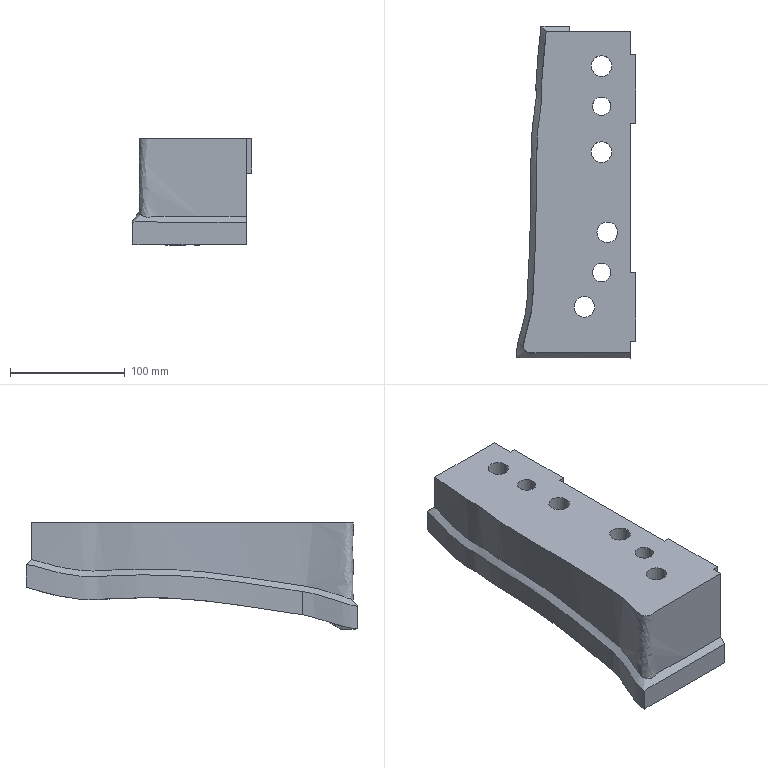Part | NX | features solid 2 | 1 solid | 42 faces | box 104.596 x 289.434 x 93.062 mm | volume 1110740 mm3 | plane 20 | cylinder 12 | spline 8 | cone 2 | commonest cylinder face diameters 18 x4 26 x4 16 x2 36 x2